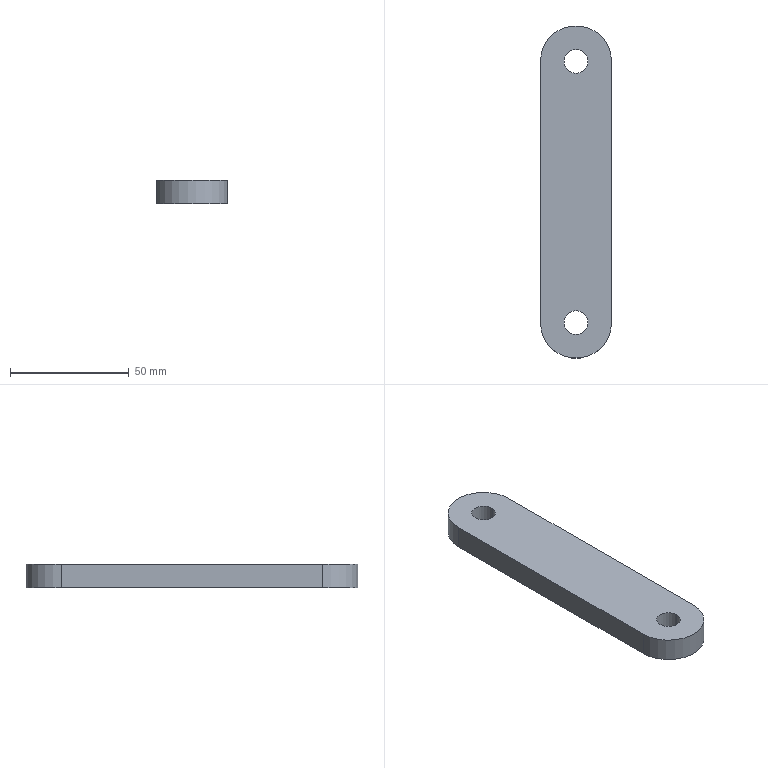Part | SolidWorks | features Extrusion 1 | 1 solid | 10 faces | box 30 x 140 x 10 mm | volume 38498 mm3 | cylinder 6 | plane 4 | commonest cylinder face diameters 10 x4 30 x2
STEP:
#1=CARTESIAN_POINT('',(-5.,110.,10.));
#2=VERTEX_POINT('',#1);
#3=CARTESIAN_POINT('',(5.,110.,10.));
#4=VERTEX_POINT('',#3);
#5=CARTESIAN_POINT('',(0.,110.,10.));
#6=DIRECTION('',(0.,0.,1.));
#7=DIRECTION('',(1.,0.,0.));
#8=AXIS2_PLACEMENT_3D('',#5,#6,#7);
#9=CIRCLE('',#8,5.);
#10=EDGE_CURVE('',#2,#4,#9,.T.);
#11=ORIENTED_EDGE('',*,*,#10,.T.);
#12=CARTESIAN_POINT('',(5.,110.,0.));
#13=VERTEX_POINT('',#12);
#14=CARTESIAN_POINT('',(5.,110.,10.));
#15=DIRECTION('',(0.,0.,-1.));
#16=VECTOR('',#15,1000.);
#17=LINE('',#14,#16);
#18=EDGE_CURVE('',#4,#13,#17,.T.);
#19=ORIENTED_EDGE('',*,*,#18,.T.);
#20=CARTESIAN_POINT('',(-5.,110.,0.));
#21=VERTEX_POINT('',#20);
#22=CARTESIAN_POINT('',(0.,110.,0.));
#23=DIRECTION('',(0.,0.,1.));
#24=DIRECTION('',(1.,0.,0.));
#25=AXIS2_PLACEMENT_3D('',#22,#23,#24);
#26=CIRCLE('',#25,5.);
#27=EDGE_CURVE('',#21,#13,#26,.T.);
#28=ORIENTED_EDGE('',*,*,#27,.F.);
#29=CARTESIAN_POINT('',(-5.,110.,10.));
#30=DIRECTION('',(0.,0.,-1.));
#31=VECTOR('',#30,1000.);
#32=LINE('',#29,#31);
#33=EDGE_CURVE('',#2,#21,#32,.T.);
#34=ORIENTED_EDGE('',*,*,#33,.F.);
#35=EDGE_LOOP('',(#11,#19,#28,#34));
#36=FACE_OUTER_BOUND('',#35,.T.);
#37=CARTESIAN_POINT('',(0.,110.,10.));
#38=DIRECTION('',(0.,0.,-1.));
#39=DIRECTION('',(-1.,0.,0.));
#40=AXIS2_PLACEMENT_3D('',#37,#38,#39);
#41=CYLINDRICAL_SURFACE('',#40,5.);
#42=ADVANCED_FACE('',(#36),#41,.F.);
#43=CARTESIAN_POINT('',(-5.,0.,10.));
#44=VERTEX_POINT('',#43);
#45=CARTESIAN_POINT('',(5.,0.,10.));
#46=VERTEX_POINT('',#45);
#47=CARTESIAN_POINT('',(0.,0.,10.));
#48=DIRECTION('',(0.,0.,1.));
#49=DIRECTION('',(1.,0.,0.));
#50=AXIS2_PLACEMENT_3D('',#47,#48,#49);
#51=CIRCLE('',#50,5.);
#52=EDGE_CURVE('',#44,#46,#51,.T.);
#53=ORIENTED_EDGE('',*,*,#52,.T.);
#54=CARTESIAN_POINT('',(5.,0.,0.));
#55=VERTEX_POINT('',#54);
#56=CARTESIAN_POINT('',(5.,0.,10.));
#57=DIRECTION('',(0.,0.,-1.));
#58=VECTOR('',#57,1000.);
#59=LINE('',#56,#58);
#60=EDGE_CURVE('',#46,#55,#59,.T.);
#61=ORIENTED_EDGE('',*,*,#60,.T.);
#62=CARTESIAN_POINT('',(-5.,0.,0.));
#63=VERTEX_POINT('',#62);
#64=CARTESIAN_POINT('',(0.,0.,0.));
#65=DIRECTION('',(0.,0.,1.));
#66=DIRECTION('',(1.,0.,0.));
#67=AXIS2_PLACEMENT_3D('',#64,#65,#66);
#68=CIRCLE('',#67,5.);
#69=EDGE_CURVE('',#63,#55,#68,.T.);
#70=ORIENTED_EDGE('',*,*,#69,.F.);
#71=CARTESIAN_POINT('',(-5.,0.,10.));
#72=DIRECTION('',(0.,0.,-1.));
#73=VECTOR('',#72,1000.);
#74=LINE('',#71,#73);
#75=EDGE_CURVE('',#44,#63,#74,.T.);
#76=ORIENTED_EDGE('',*,*,#75,.F.);
#77=EDGE_LOOP('',(#53,#61,#70,#76));
#78=FACE_OUTER_BOUND('',#77,.T.);
#79=CARTESIAN_POINT('',(0.,0.,10.));
#80=DIRECTION('',(0.,0.,-1.));
#81=DIRECTION('',(-1.,0.,0.));
#82=AXIS2_PLACEMENT_3D('',#79,#80,#81);
#83=CYLINDRICAL_SURFACE('',#82,5.);
#84=ADVANCED_FACE('',(#78),#83,.F.);
#85=ORIENTED_EDGE('',*,*,#52,.F.);
#86=CARTESIAN_POINT('',(0.,0.,10.));
#87=DIRECTION('',(0.,0.,1.));
#88=DIRECTION('',(1.,0.,0.));
#89=AXIS2_PLACEMENT_3D('',#86,#87,#88);
#90=CIRCLE('',#89,5.);
#91=EDGE_CURVE('',#46,#44,#90,.T.);
#92=ORIENTED_EDGE('',*,*,#91,.F.);
#93=EDGE_LOOP('',(#85,#92));
#94=FACE_BOUND('',#93,.T.);
#95=CARTESIAN_POINT('',(-15.,0.,10.));
#96=VERTEX_POINT('',#95);
#97=CARTESIAN_POINT('',(15.,0.,10.));
#98=VERTEX_POINT('',#97);
#99=CARTESIAN_POINT('',(0.,0.,10.));
#100=DIRECTION('',(0.,0.,1.));
#101=DIRECTION('',(1.,0.,0.));
#102=AXIS2_PLACEMENT_3D('',#99,#100,#101);
#103=CIRCLE('',#102,15.);
#104=EDGE_CURVE('',#96,#98,#103,.T.);
#105=ORIENTED_EDGE('',*,*,#104,.T.);
#106=CARTESIAN_POINT('',(15.,110.,10.));
#107=VERTEX_POINT('',#106);
#108=CARTESIAN_POINT('',(15.,0.,10.));
#109=DIRECTION('',(0.,1.,0.));
#110=VECTOR('',#109,1000.);
#111=LINE('',#108,#110);
#112=EDGE_CURVE('',#98,#107,#111,.T.);
#113=ORIENTED_EDGE('',*,*,#112,.T.);
#114=CARTESIAN_POINT('',(-15.,110.,10.));
#115=VERTEX_POINT('',#114);
#116=CARTESIAN_POINT('',(0.,110.,10.));
#117=DIRECTION('',(0.,0.,1.));
#118=DIRECTION('',(1.,0.,0.));
#119=AXIS2_PLACEMENT_3D('',#116,#117,#118);
#120=CIRCLE('',#119,15.);
#121=EDGE_CURVE('',#107,#115,#120,.T.);
#122=ORIENTED_EDGE('',*,*,#121,.T.);
#123=CARTESIAN_POINT('',(-15.,0.,10.));
#124=DIRECTION('',(0.,-1.,0.));
#125=VECTOR('',#124,1000.);
#126=LINE('',#123,#125);
#127=EDGE_CURVE('',#115,#96,#126,.T.);
#128=ORIENTED_EDGE('',*,*,#127,.T.);
#129=EDGE_LOOP('',(#105,#113,#122,#128));
#130=FACE_OUTER_BOUND('',#129,.T.);
#131=ORIENTED_EDGE('',*,*,#10,.F.);
#132=CARTESIAN_POINT('',(0.,110.,10.));
#133=DIRECTION('',(0.,0.,1.));
#134=DIRECTION('',(1.,0.,0.));
#135=AXIS2_PLACEMENT_3D('',#132,#133,#134);
#136=CIRCLE('',#135,5.);
#137=EDGE_CURVE('',#4,#2,#136,.T.);
#138=ORIENTED_EDGE('',*,*,#137,.F.);
#139=EDGE_LOOP('',(#131,#138));
#140=FACE_BOUND('',#139,.T.);
#141=CARTESIAN_POINT('',(0.,0.,10.));
#142=DIRECTION('',(0.,0.,1.));
#143=DIRECTION('',(1.,0.,0.));
#144=AXIS2_PLACEMENT_3D('',#141,#142,#143);
#145=PLANE('',#144);
#146=ADVANCED_FACE('',(#94,#130,#140),#145,.T.);
#147=CARTESIAN_POINT('',(-15.,0.,0.));
#148=VERTEX_POINT('',#147);
#149=CARTESIAN_POINT('',(15.,0.,0.));
#150=VERTEX_POINT('',#149);
#151=CARTESIAN_POINT('',(0.,0.,0.));
#152=DIRECTION('',(0.,0.,1.));
#153=DIRECTION('',(1.,0.,0.));
#154=AXIS2_PLACEMENT_3D('',#151,#152,#153);
#155=CIRCLE('',#154,15.);
#156=EDGE_CURVE('',#148,#150,#155,.T.);
#157=ORIENTED_EDGE('',*,*,#156,.F.);
#158=CARTESIAN_POINT('',(-15.,110.,0.));
#159=VERTEX_POINT('',#158);
#160=CARTESIAN_POINT('',(-15.,0.,0.));
#161=DIRECTION('',(0.,-1.,0.));
#162=VECTOR('',#161,1000.);
#163=LINE('',#160,#162);
#164=EDGE_CURVE('',#159,#148,#163,.T.);
#165=ORIENTED_EDGE('',*,*,#164,.F.);
#166=CARTESIAN_POINT('',(15.,110.,0.));
#167=VERTEX_POINT('',#166);
#168=CARTESIAN_POINT('',(0.,110.,0.));
#169=DIRECTION('',(0.,0.,1.));
#170=DIRECTION('',(1.,0.,0.));
#171=AXIS2_PLACEMENT_3D('',#168,#169,#170);
#172=CIRCLE('',#171,15.);
#173=EDGE_CURVE('',#167,#159,#172,.T.);
#174=ORIENTED_EDGE('',*,*,#173,.F.);
#175=CARTESIAN_POINT('',(15.,0.,0.));
#176=DIRECTION('',(0.,1.,0.));
#177=VECTOR('',#176,1000.);
#178=LINE('',#175,#177);
#179=EDGE_CURVE('',#150,#167,#178,.T.);
#180=ORIENTED_EDGE('',*,*,#179,.F.);
#181=EDGE_LOOP('',(#157,#165,#174,#180));
#182=FACE_OUTER_BOUND('',#181,.T.);
#183=ORIENTED_EDGE('',*,*,#69,.T.);
#184=CARTESIAN_POINT('',(0.,0.,0.));
#185=DIRECTION('',(0.,0.,1.));
#186=DIRECTION('',(1.,0.,0.));
#187=AXIS2_PLACEMENT_3D('',#184,#185,#186);
#188=CIRCLE('',#187,5.);
#189=EDGE_CURVE('',#55,#63,#188,.T.);
#190=ORIENTED_EDGE('',*,*,#189,.T.);
#191=EDGE_LOOP('',(#183,#190));
#192=FACE_BOUND('',#191,.T.);
#193=ORIENTED_EDGE('',*,*,#27,.T.);
#194=CARTESIAN_POINT('',(0.,110.,0.));
#195=DIRECTION('',(0.,0.,1.));
#196=DIRECTION('',(1.,0.,0.));
#197=AXIS2_PLACEMENT_3D('',#194,#195,#196);
#198=CIRCLE('',#197,5.);
#199=EDGE_CURVE('',#13,#21,#198,.T.);
#200=ORIENTED_EDGE('',*,*,#199,.T.);
#201=EDGE_LOOP('',(#193,#200));
#202=FACE_BOUND('',#201,.T.);
#203=CARTESIAN_POINT('',(0.,0.,0.));
#204=DIRECTION('',(0.,0.,1.));
#205=DIRECTION('',(1.,0.,0.));
#206=AXIS2_PLACEMENT_3D('',#203,#204,#205);
#207=PLANE('',#206);
#208=ADVANCED_FACE('',(#182,#192,#202),#207,.F.);
#209=ORIENTED_EDGE('',*,*,#156,.T.);
#210=CARTESIAN_POINT('',(15.,0.,10.));
#211=DIRECTION('',(0.,0.,-1.));
#212=VECTOR('',#211,1000.);
#213=LINE('',#210,#212);
#214=EDGE_CURVE('',#98,#150,#213,.T.);
#215=ORIENTED_EDGE('',*,*,#214,.F.);
#216=ORIENTED_EDGE('',*,*,#104,.F.);
#217=CARTESIAN_POINT('',(-15.,0.,10.));
#218=DIRECTION('',(0.,0.,-1.));
#219=VECTOR('',#218,1000.);
#220=LINE('',#217,#219);
#221=EDGE_CURVE('',#96,#148,#220,.T.);
#222=ORIENTED_EDGE('',*,*,#221,.T.);
#223=EDGE_LOOP('',(#209,#215,#216,#222));
#224=FACE_OUTER_BOUND('',#223,.T.);
#225=CARTESIAN_POINT('',(0.,0.,10.));
#226=DIRECTION('',(0.,0.,-1.));
#227=DIRECTION('',(-1.,0.,0.));
#228=AXIS2_PLACEMENT_3D('',#225,#226,#227);
#229=CYLINDRICAL_SURFACE('',#228,15.);
#230=ADVANCED_FACE('',(#224),#229,.T.);
#231=ORIENTED_EDGE('',*,*,#179,.T.);
#232=CARTESIAN_POINT('',(15.,110.,10.));
#233=DIRECTION('',(0.,0.,-1.));
#234=VECTOR('',#233,1000.);
#235=LINE('',#232,#234);
#236=EDGE_CURVE('',#107,#167,#235,.T.);
#237=ORIENTED_EDGE('',*,*,#236,.F.);
#238=ORIENTED_EDGE('',*,*,#112,.F.);
#239=ORIENTED_EDGE('',*,*,#214,.T.);
#240=EDGE_LOOP('',(#231,#237,#238,#239));
#241=FACE_OUTER_BOUND('',#240,.T.);
#242=CARTESIAN_POINT('',(15.,0.,10.));
#243=DIRECTION('',(-1.,0.,0.));
#244=DIRECTION('',(0.,0.,1.));
#245=AXIS2_PLACEMENT_3D('',#242,#243,#244);
#246=PLANE('',#245);
#247=ADVANCED_FACE('',(#241),#246,.F.);
#248=ORIENTED_EDGE('',*,*,#173,.T.);
#249=CARTESIAN_POINT('',(-15.,110.,10.));
#250=DIRECTION('',(0.,0.,-1.));
#251=VECTOR('',#250,1000.);
#252=LINE('',#249,#251);
#253=EDGE_CURVE('',#115,#159,#252,.T.);
#254=ORIENTED_EDGE('',*,*,#253,.F.);
#255=ORIENTED_EDGE('',*,*,#121,.F.);
#256=ORIENTED_EDGE('',*,*,#236,.T.);
#257=EDGE_LOOP('',(#248,#254,#255,#256));
#258=FACE_OUTER_BOUND('',#257,.T.);
#259=CARTESIAN_POINT('',(0.,110.,10.));
#260=DIRECTION('',(0.,0.,-1.));
#261=DIRECTION('',(-1.,0.,0.));
#262=AXIS2_PLACEMENT_3D('',#259,#260,#261);
#263=CYLINDRICAL_SURFACE('',#262,15.);
#264=ADVANCED_FACE('',(#258),#263,.T.);
#265=ORIENTED_EDGE('',*,*,#164,.T.);
#266=ORIENTED_EDGE('',*,*,#221,.F.);
#267=ORIENTED_EDGE('',*,*,#127,.F.);
#268=ORIENTED_EDGE('',*,*,#253,.T.);
#269=EDGE_LOOP('',(#265,#266,#267,#268));
#270=FACE_OUTER_BOUND('',#269,.T.);
#271=CARTESIAN_POINT('',(-15.,0.,10.));
#272=DIRECTION('',(1.,0.,0.));
#273=DIRECTION('',(0.,0.,-1.));
#274=AXIS2_PLACEMENT_3D('',#271,#272,#273);
#275=PLANE('',#274);
#276=ADVANCED_FACE('',(#270),#275,.F.);
#277=ORIENTED_EDGE('',*,*,#60,.F.);
#278=ORIENTED_EDGE('',*,*,#91,.T.);
#279=ORIENTED_EDGE('',*,*,#75,.T.);
#280=ORIENTED_EDGE('',*,*,#189,.F.);
#281=EDGE_LOOP('',(#277,#278,#279,#280));
#282=FACE_OUTER_BOUND('',#281,.T.);
#283=CARTESIAN_POINT('',(0.,0.,10.));
#284=DIRECTION('',(0.,0.,-1.));
#285=DIRECTION('',(-1.,0.,0.));
#286=AXIS2_PLACEMENT_3D('',#283,#284,#285);
#287=CYLINDRICAL_SURFACE('',#286,5.);
#288=ADVANCED_FACE('',(#282),#287,.F.);
#289=ORIENTED_EDGE('',*,*,#18,.F.);
#290=ORIENTED_EDGE('',*,*,#137,.T.);
#291=ORIENTED_EDGE('',*,*,#33,.T.);
#292=ORIENTED_EDGE('',*,*,#199,.F.);
#293=EDGE_LOOP('',(#289,#290,#291,#292));
#294=FACE_OUTER_BOUND('',#293,.T.);
#295=CARTESIAN_POINT('',(0.,110.,10.));
#296=DIRECTION('',(0.,0.,-1.));
#297=DIRECTION('',(-1.,0.,0.));
#298=AXIS2_PLACEMENT_3D('',#295,#296,#297);
#299=CYLINDRICAL_SURFACE('',#298,5.);
#300=ADVANCED_FACE('',(#294),#299,.F.);
#301=CLOSED_SHELL('',(#42,#84,#146,#208,#230,#247,#264,#276,#288,#300));
#302=MANIFOLD_SOLID_BREP('',#301);
#303=CARTESIAN_POINT('',(0.,0.,0.));
#304=DIRECTION('',(0.,0.,1.));
#305=DIRECTION('',(1.,0.,0.));
#306=AXIS2_PLACEMENT_3D('',#303,#304,#305);
#307=(LENGTH_UNIT()NAMED_UNIT(*)SI_UNIT(.MILLI.,.METRE.));
#308=UNCERTAINTY_MEASURE_WITH_UNIT(LENGTH_MEASURE(0.00001),#307,'','');
#309=(NAMED_UNIT(*)PLANE_ANGLE_UNIT()SI_UNIT($,.RADIAN.));
#310=(NAMED_UNIT(*)SI_UNIT($,.STERADIAN.)SOLID_ANGLE_UNIT());
#311=(GEOMETRIC_REPRESENTATION_CONTEXT(3)GLOBAL_UNCERTAINTY_ASSIGNED_CONTEXT((#308))GLOBAL_UNIT_ASSIGNED_CONTEXT((#307,#309,#310))REPRESENTATION_CONTEXT('',''));
#312=ADVANCED_BREP_SHAPE_REPRESENTATION('',(#302,#306),#311);